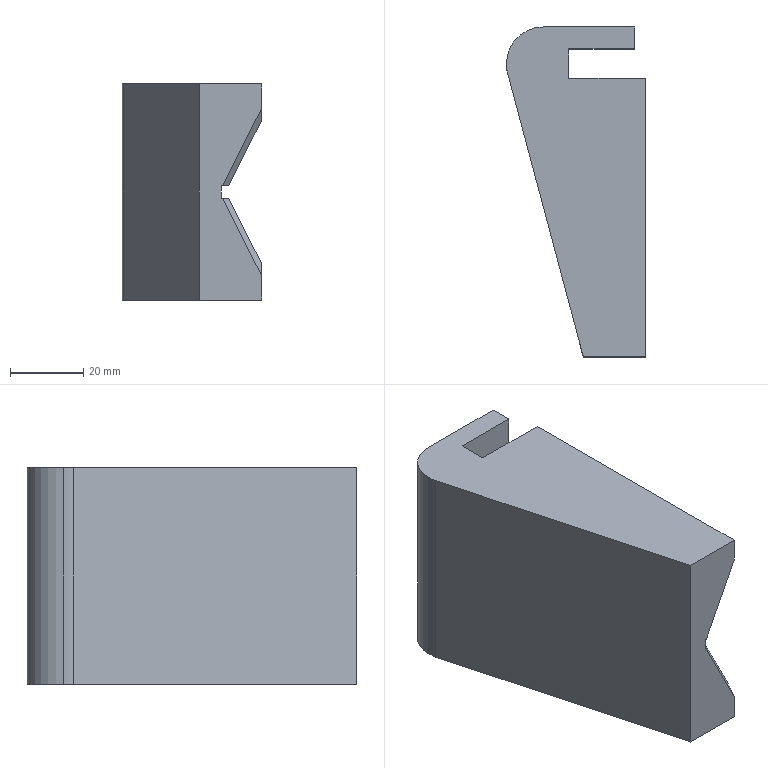Part | SolidWorks | features ICE 5, Extrusion 1 | 1 solid | 189 faces | box 37.984 x 90 x 59 mm | volume 121920 mm3 | plane 186 | cylinder 3 | commonest cylinder face diameters 20 x2 28 x1